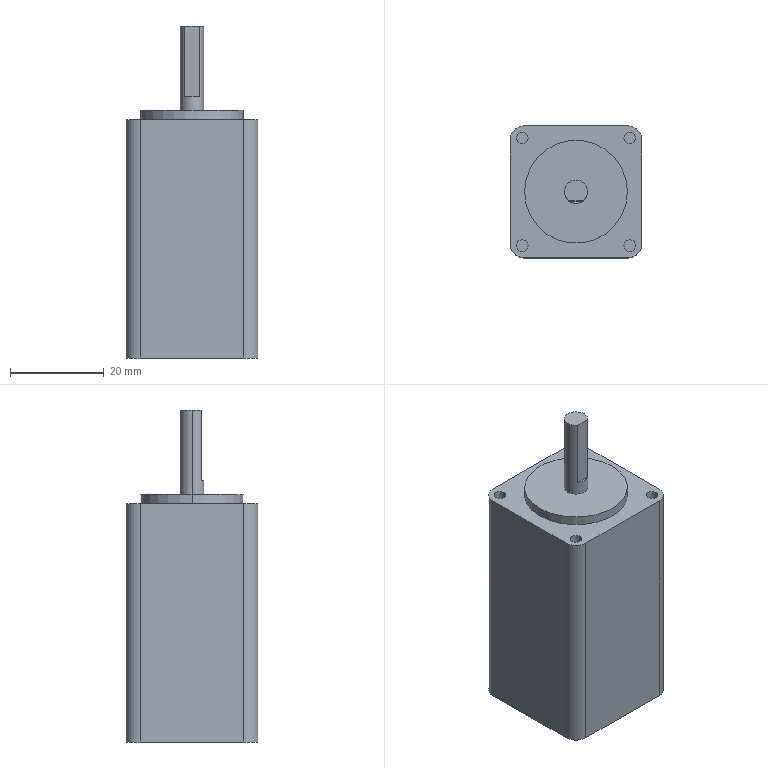Part | SolidWorks | features MBimport 1 | 1 solid | 30 faces | box 28.2 x 28.2 x 71 mm | volume 41213 mm3 | cylinder 16 | plane 14 | commonest cylinder face diameters 2.5 x8 6 x4 5 x2 22 x2
STEP:
#1=CARTESIAN_POINT('',(2.5,0.,71.));
#2=VERTEX_POINT('',#1);
#3=CARTESIAN_POINT('',(-2.5,0.,71.));
#4=VERTEX_POINT('',#3);
#5=CARTESIAN_POINT('',(0.,0.,71.));
#6=DIRECTION('',(0.,0.,1.));
#7=DIRECTION('',(1.,0.,0.));
#8=AXIS2_PLACEMENT_3D('',#5,#6,#7);
#9=CIRCLE('',#8,2.5);
#10=EDGE_CURVE('',#2,#4,#9,.T.);
#11=ORIENTED_EDGE('',*,*,#10,.F.);
#12=CARTESIAN_POINT('',(2.5,0.,53.));
#13=VERTEX_POINT('',#12);
#14=CARTESIAN_POINT('',(2.5,0.,71.));
#15=DIRECTION('',(0.,0.,-1.));
#16=VECTOR('',#15,1000.);
#17=LINE('',#14,#16);
#18=EDGE_CURVE('',#2,#13,#17,.T.);
#19=ORIENTED_EDGE('',*,*,#18,.T.);
#20=CARTESIAN_POINT('',(-2.5,0.,53.));
#21=VERTEX_POINT('',#20);
#22=CARTESIAN_POINT('',(0.,0.,53.));
#23=DIRECTION('',(0.,0.,1.));
#24=DIRECTION('',(1.,0.,0.));
#25=AXIS2_PLACEMENT_3D('',#22,#23,#24);
#26=CIRCLE('',#25,2.5);
#27=EDGE_CURVE('',#13,#21,#26,.T.);
#28=ORIENTED_EDGE('',*,*,#27,.T.);
#29=CARTESIAN_POINT('',(-2.5,0.,71.));
#30=DIRECTION('',(0.,0.,-1.));
#31=VECTOR('',#30,1000.);
#32=LINE('',#29,#31);
#33=EDGE_CURVE('',#4,#21,#32,.T.);
#34=ORIENTED_EDGE('',*,*,#33,.F.);
#35=EDGE_LOOP('',(#11,#19,#28,#34));
#36=FACE_OUTER_BOUND('',#35,.T.);
#37=CARTESIAN_POINT('',(0.,0.,71.));
#38=DIRECTION('',(0.,0.,-1.));
#39=DIRECTION('',(-1.,0.,0.));
#40=AXIS2_PLACEMENT_3D('',#37,#38,#39);
#41=CYLINDRICAL_SURFACE('',#40,2.5);
#42=ADVANCED_FACE('',(#36),#41,.T.);
#43=CARTESIAN_POINT('',(11.,0.,53.));
#44=VERTEX_POINT('',#43);
#45=CARTESIAN_POINT('',(-11.,0.,53.));
#46=VERTEX_POINT('',#45);
#47=CARTESIAN_POINT('',(0.,0.,53.));
#48=DIRECTION('',(0.,0.,1.));
#49=DIRECTION('',(1.,0.,0.));
#50=AXIS2_PLACEMENT_3D('',#47,#48,#49);
#51=CIRCLE('',#50,11.);
#52=EDGE_CURVE('',#44,#46,#51,.T.);
#53=ORIENTED_EDGE('',*,*,#52,.F.);
#54=CARTESIAN_POINT('',(11.,0.,51.));
#55=VERTEX_POINT('',#54);
#56=CARTESIAN_POINT('',(11.,0.,53.));
#57=DIRECTION('',(0.,0.,-1.));
#58=VECTOR('',#57,1000.);
#59=LINE('',#56,#58);
#60=EDGE_CURVE('',#44,#55,#59,.T.);
#61=ORIENTED_EDGE('',*,*,#60,.T.);
#62=CARTESIAN_POINT('',(-11.,0.,51.));
#63=VERTEX_POINT('',#62);
#64=CARTESIAN_POINT('',(0.,0.,51.));
#65=DIRECTION('',(0.,0.,1.));
#66=DIRECTION('',(-1.,0.,0.));
#67=AXIS2_PLACEMENT_3D('',#64,#65,#66);
#68=CIRCLE('',#67,11.);
#69=EDGE_CURVE('',#55,#63,#68,.T.);
#70=ORIENTED_EDGE('',*,*,#69,.T.);
#71=CARTESIAN_POINT('',(-11.,0.,53.));
#72=DIRECTION('',(0.,0.,-1.));
#73=VECTOR('',#72,1000.);
#74=LINE('',#71,#73);
#75=EDGE_CURVE('',#46,#63,#74,.T.);
#76=ORIENTED_EDGE('',*,*,#75,.F.);
#77=EDGE_LOOP('',(#53,#61,#70,#76));
#78=FACE_OUTER_BOUND('',#77,.T.);
#79=CARTESIAN_POINT('',(0.,0.,53.));
#80=DIRECTION('',(0.,0.,-1.));
#81=DIRECTION('',(-1.,0.,0.));
#82=AXIS2_PLACEMENT_3D('',#79,#80,#81);
#83=CYLINDRICAL_SURFACE('',#82,11.);
#84=ADVANCED_FACE('',(#78),#83,.T.);
#85=CARTESIAN_POINT('',(10.25,-11.5,48.5));
#86=VERTEX_POINT('',#85);
#87=CARTESIAN_POINT('',(12.75,-11.5,48.5));
#88=VERTEX_POINT('',#87);
#89=CARTESIAN_POINT('',(11.5,-11.5,48.5));
#90=DIRECTION('',(0.,0.,1.));
#91=DIRECTION('',(1.,0.,0.));
#92=AXIS2_PLACEMENT_3D('',#89,#90,#91);
#93=CIRCLE('',#92,1.25);
#94=EDGE_CURVE('',#86,#88,#93,.T.);
#95=ORIENTED_EDGE('',*,*,#94,.F.);
#96=CARTESIAN_POINT('',(10.25,-11.5,51.));
#97=VERTEX_POINT('',#96);
#98=CARTESIAN_POINT('',(10.25,-11.5,48.5));
#99=DIRECTION('',(0.,0.,1.));
#100=VECTOR('',#99,1000.);
#101=LINE('',#98,#100);
#102=EDGE_CURVE('',#86,#97,#101,.T.);
#103=ORIENTED_EDGE('',*,*,#102,.T.);
#104=CARTESIAN_POINT('',(12.75,-11.5,51.));
#105=VERTEX_POINT('',#104);
#106=CARTESIAN_POINT('',(11.5,-11.5,51.));
#107=DIRECTION('',(0.,0.,1.));
#108=DIRECTION('',(1.,0.,0.));
#109=AXIS2_PLACEMENT_3D('',#106,#107,#108);
#110=CIRCLE('',#109,1.25);
#111=EDGE_CURVE('',#97,#105,#110,.T.);
#112=ORIENTED_EDGE('',*,*,#111,.T.);
#113=CARTESIAN_POINT('',(12.75,-11.5,48.5));
#114=DIRECTION('',(0.,0.,1.));
#115=VECTOR('',#114,1000.);
#116=LINE('',#113,#115);
#117=EDGE_CURVE('',#88,#105,#116,.T.);
#118=ORIENTED_EDGE('',*,*,#117,.F.);
#119=EDGE_LOOP('',(#95,#103,#112,#118));
#120=FACE_OUTER_BOUND('',#119,.T.);
#121=CARTESIAN_POINT('',(11.5,-11.5,48.5));
#122=DIRECTION('',(0.,0.,1.));
#123=DIRECTION('',(1.,0.,0.));
#124=AXIS2_PLACEMENT_3D('',#121,#122,#123);
#125=CYLINDRICAL_SURFACE('',#124,1.25);
#126=ADVANCED_FACE('',(#120),#125,.F.);
#127=CARTESIAN_POINT('',(-12.75,-11.5,48.5));
#128=VERTEX_POINT('',#127);
#129=CARTESIAN_POINT('',(-10.25,-11.5,48.5));
#130=VERTEX_POINT('',#129);
#131=CARTESIAN_POINT('',(-11.5,-11.5,48.5));
#132=DIRECTION('',(0.,0.,1.));
#133=DIRECTION('',(1.,0.,0.));
#134=AXIS2_PLACEMENT_3D('',#131,#132,#133);
#135=CIRCLE('',#134,1.25);
#136=EDGE_CURVE('',#128,#130,#135,.T.);
#137=ORIENTED_EDGE('',*,*,#136,.F.);
#138=CARTESIAN_POINT('',(-12.75,-11.5,51.));
#139=VERTEX_POINT('',#138);
#140=CARTESIAN_POINT('',(-12.75,-11.5,48.5));
#141=DIRECTION('',(0.,0.,1.));
#142=VECTOR('',#141,1000.);
#143=LINE('',#140,#142);
#144=EDGE_CURVE('',#128,#139,#143,.T.);
#145=ORIENTED_EDGE('',*,*,#144,.T.);
#146=CARTESIAN_POINT('',(-10.25,-11.5,51.));
#147=VERTEX_POINT('',#146);
#148=CARTESIAN_POINT('',(-11.5,-11.5,51.));
#149=DIRECTION('',(0.,0.,1.));
#150=DIRECTION('',(1.,0.,0.));
#151=AXIS2_PLACEMENT_3D('',#148,#149,#150);
#152=CIRCLE('',#151,1.25);
#153=EDGE_CURVE('',#139,#147,#152,.T.);
#154=ORIENTED_EDGE('',*,*,#153,.T.);
#155=CARTESIAN_POINT('',(-10.25,-11.5,48.5));
#156=DIRECTION('',(0.,0.,1.));
#157=VECTOR('',#156,1000.);
#158=LINE('',#155,#157);
#159=EDGE_CURVE('',#130,#147,#158,.T.);
#160=ORIENTED_EDGE('',*,*,#159,.F.);
#161=EDGE_LOOP('',(#137,#145,#154,#160));
#162=FACE_OUTER_BOUND('',#161,.T.);
#163=CARTESIAN_POINT('',(-11.5,-11.5,48.5));
#164=DIRECTION('',(0.,0.,1.));
#165=DIRECTION('',(1.,0.,0.));
#166=AXIS2_PLACEMENT_3D('',#163,#164,#165);
#167=CYLINDRICAL_SURFACE('',#166,1.25);
#168=ADVANCED_FACE('',(#162),#167,.F.);
#169=CARTESIAN_POINT('',(10.25,11.5,48.5));
#170=VERTEX_POINT('',#169);
#171=CARTESIAN_POINT('',(12.75,11.5,48.5));
#172=VERTEX_POINT('',#171);
#173=CARTESIAN_POINT('',(11.5,11.5,48.5));
#174=DIRECTION('',(0.,0.,1.));
#175=DIRECTION('',(1.,0.,0.));
#176=AXIS2_PLACEMENT_3D('',#173,#174,#175);
#177=CIRCLE('',#176,1.25);
#178=EDGE_CURVE('',#170,#172,#177,.T.);
#179=ORIENTED_EDGE('',*,*,#178,.F.);
#180=CARTESIAN_POINT('',(10.25,11.5,51.));
#181=VERTEX_POINT('',#180);
#182=CARTESIAN_POINT('',(10.25,11.5,48.5));
#183=DIRECTION('',(0.,0.,1.));
#184=VECTOR('',#183,1000.);
#185=LINE('',#182,#184);
#186=EDGE_CURVE('',#170,#181,#185,.T.);
#187=ORIENTED_EDGE('',*,*,#186,.T.);
#188=CARTESIAN_POINT('',(12.75,11.5,51.));
#189=VERTEX_POINT('',#188);
#190=CARTESIAN_POINT('',(11.5,11.5,51.));
#191=DIRECTION('',(0.,0.,1.));
#192=DIRECTION('',(1.,0.,0.));
#193=AXIS2_PLACEMENT_3D('',#190,#191,#192);
#194=CIRCLE('',#193,1.25);
#195=EDGE_CURVE('',#181,#189,#194,.T.);
#196=ORIENTED_EDGE('',*,*,#195,.T.);
#197=CARTESIAN_POINT('',(12.75,11.5,48.5));
#198=DIRECTION('',(0.,0.,1.));
#199=VECTOR('',#198,1000.);
#200=LINE('',#197,#199);
#201=EDGE_CURVE('',#172,#189,#200,.T.);
#202=ORIENTED_EDGE('',*,*,#201,.F.);
#203=EDGE_LOOP('',(#179,#187,#196,#202));
#204=FACE_OUTER_BOUND('',#203,.T.);
#205=CARTESIAN_POINT('',(11.5,11.5,48.5));
#206=DIRECTION('',(0.,0.,1.));
#207=DIRECTION('',(1.,0.,0.));
#208=AXIS2_PLACEMENT_3D('',#205,#206,#207);
#209=CYLINDRICAL_SURFACE('',#208,1.25);
#210=ADVANCED_FACE('',(#204),#209,.F.);
#211=CARTESIAN_POINT('',(-12.75,11.5,48.5));
#212=VERTEX_POINT('',#211);
#213=CARTESIAN_POINT('',(-10.25,11.5,48.5));
#214=VERTEX_POINT('',#213);
#215=CARTESIAN_POINT('',(-11.5,11.5,48.5));
#216=DIRECTION('',(0.,0.,1.));
#217=DIRECTION('',(1.,0.,0.));
#218=AXIS2_PLACEMENT_3D('',#215,#216,#217);
#219=CIRCLE('',#218,1.25);
#220=EDGE_CURVE('',#212,#214,#219,.T.);
#221=ORIENTED_EDGE('',*,*,#220,.F.);
#222=CARTESIAN_POINT('',(-12.75,11.5,51.));
#223=VERTEX_POINT('',#222);
#224=CARTESIAN_POINT('',(-12.75,11.5,48.5));
#225=DIRECTION('',(0.,0.,1.));
#226=VECTOR('',#225,1000.);
#227=LINE('',#224,#226);
#228=EDGE_CURVE('',#212,#223,#227,.T.);
#229=ORIENTED_EDGE('',*,*,#228,.T.);
#230=CARTESIAN_POINT('',(-10.25,11.5,51.));
#231=VERTEX_POINT('',#230);
#232=CARTESIAN_POINT('',(-11.5,11.5,51.));
#233=DIRECTION('',(0.,0.,1.));
#234=DIRECTION('',(1.,0.,0.));
#235=AXIS2_PLACEMENT_3D('',#232,#233,#234);
#236=CIRCLE('',#235,1.25);
#237=EDGE_CURVE('',#223,#231,#236,.T.);
#238=ORIENTED_EDGE('',*,*,#237,.T.);
#239=CARTESIAN_POINT('',(-10.25,11.5,48.5));
#240=DIRECTION('',(0.,0.,1.));
#241=VECTOR('',#240,1000.);
#242=LINE('',#239,#241);
#243=EDGE_CURVE('',#214,#231,#242,.T.);
#244=ORIENTED_EDGE('',*,*,#243,.F.);
#245=EDGE_LOOP('',(#221,#229,#238,#244));
#246=FACE_OUTER_BOUND('',#245,.T.);
#247=CARTESIAN_POINT('',(-11.5,11.5,48.5));
#248=DIRECTION('',(0.,0.,1.));
#249=DIRECTION('',(1.,0.,0.));
#250=AXIS2_PLACEMENT_3D('',#247,#248,#249);
#251=CYLINDRICAL_SURFACE('',#250,1.25);
#252=ADVANCED_FACE('',(#246),#251,.F.);
#253=CARTESIAN_POINT('',(0.,0.,53.));
#254=DIRECTION('',(0.,0.,1.));
#255=DIRECTION('',(1.,0.,0.));
#256=AXIS2_PLACEMENT_3D('',#253,#254,#255);
#257=CIRCLE('',#256,11.);
#258=EDGE_CURVE('',#46,#44,#257,.T.);
#259=ORIENTED_EDGE('',*,*,#258,.T.);
#260=ORIENTED_EDGE('',*,*,#52,.T.);
#261=EDGE_LOOP('',(#259,#260));
#262=FACE_OUTER_BOUND('',#261,.T.);
#263=CARTESIAN_POINT('',(0.,0.,53.));
#264=DIRECTION('',(0.,0.,1.));
#265=DIRECTION('',(1.,0.,0.));
#266=AXIS2_PLACEMENT_3D('',#263,#264,#265);
#267=CIRCLE('',#266,2.5);
#268=EDGE_CURVE('',#21,#13,#267,.T.);
#269=ORIENTED_EDGE('',*,*,#268,.F.);
#270=ORIENTED_EDGE('',*,*,#27,.F.);
#271=EDGE_LOOP('',(#269,#270));
#272=FACE_BOUND('',#271,.T.);
#273=CARTESIAN_POINT('',(0.,0.,53.));
#274=DIRECTION('',(0.,0.,1.));
#275=DIRECTION('',(1.,0.,0.));
#276=AXIS2_PLACEMENT_3D('',#273,#274,#275);
#277=PLANE('',#276);
#278=ADVANCED_FACE('',(#262,#272),#277,.T.);
#279=CARTESIAN_POINT('',(-14.1,11.1,51.));
#280=VERTEX_POINT('',#279);
#281=CARTESIAN_POINT('',(-14.1,-11.1,51.));
#282=VERTEX_POINT('',#281);
#283=CARTESIAN_POINT('',(-14.1,-14.1,51.));
#284=DIRECTION('',(0.,-1.,0.));
#285=VECTOR('',#284,1000.);
#286=LINE('',#283,#285);
#287=EDGE_CURVE('',#280,#282,#286,.T.);
#288=ORIENTED_EDGE('',*,*,#287,.T.);
#289=CARTESIAN_POINT('',(-11.1,-14.1,51.));
#290=VERTEX_POINT('',#289);
#291=CARTESIAN_POINT('',(-11.1,-11.1,51.));
#292=DIRECTION('',(0.,0.,1.));
#293=DIRECTION('',(-1.,0.,0.));
#294=AXIS2_PLACEMENT_3D('',#291,#292,#293);
#295=CIRCLE('',#294,3.);
#296=EDGE_CURVE('',#282,#290,#295,.T.);
#297=ORIENTED_EDGE('',*,*,#296,.T.);
#298=CARTESIAN_POINT('',(11.1,-14.1,51.));
#299=VERTEX_POINT('',#298);
#300=CARTESIAN_POINT('',(-14.1,-14.1,51.));
#301=DIRECTION('',(1.,0.,0.));
#302=VECTOR('',#301,1000.);
#303=LINE('',#300,#302);
#304=EDGE_CURVE('',#290,#299,#303,.T.);
#305=ORIENTED_EDGE('',*,*,#304,.T.);
#306=CARTESIAN_POINT('',(14.1,-11.1,51.));
#307=VERTEX_POINT('',#306);
#308=CARTESIAN_POINT('',(11.1,-11.1,51.));
#309=DIRECTION('',(0.,0.,1.));
#310=DIRECTION('',(-1.,0.,0.));
#311=AXIS2_PLACEMENT_3D('',#308,#309,#310);
#312=CIRCLE('',#311,3.);
#313=EDGE_CURVE('',#299,#307,#312,.T.);
#314=ORIENTED_EDGE('',*,*,#313,.T.);
#315=CARTESIAN_POINT('',(14.1,11.1,51.));
#316=VERTEX_POINT('',#315);
#317=CARTESIAN_POINT('',(14.1,-14.1,51.));
#318=DIRECTION('',(0.,1.,0.));
#319=VECTOR('',#318,1000.);
#320=LINE('',#317,#319);
#321=EDGE_CURVE('',#307,#316,#320,.T.);
#322=ORIENTED_EDGE('',*,*,#321,.T.);
#323=CARTESIAN_POINT('',(11.1,14.1,51.));
#324=VERTEX_POINT('',#323);
#325=CARTESIAN_POINT('',(11.1,11.1,51.));
#326=DIRECTION('',(0.,0.,1.));
#327=DIRECTION('',(-1.,0.,0.));
#328=AXIS2_PLACEMENT_3D('',#325,#326,#327);
#329=CIRCLE('',#328,3.);
#330=EDGE_CURVE('',#316,#324,#329,.T.);
#331=ORIENTED_EDGE('',*,*,#330,.T.);
#332=CARTESIAN_POINT('',(-11.1,14.1,51.));
#333=VERTEX_POINT('',#332);
#334=CARTESIAN_POINT('',(-14.1,14.1,51.));
#335=DIRECTION('',(-1.,0.,0.));
#336=VECTOR('',#335,1000.);
#337=LINE('',#334,#336);
#338=EDGE_CURVE('',#324,#333,#337,.T.);
#339=ORIENTED_EDGE('',*,*,#338,.T.);
#340=CARTESIAN_POINT('',(-11.1,11.1,51.));
#341=DIRECTION('',(0.,0.,1.));
#342=DIRECTION('',(-1.,0.,0.));
#343=AXIS2_PLACEMENT_3D('',#340,#341,#342);
#344=CIRCLE('',#343,3.);
#345=EDGE_CURVE('',#333,#280,#344,.T.);
#346=ORIENTED_EDGE('',*,*,#345,.T.);
#347=EDGE_LOOP('',(#288,#297,#305,#314,#322,#331,#339,#346));
#348=FACE_OUTER_BOUND('',#347,.T.);
#349=CARTESIAN_POINT('',(-11.5,11.5,51.));
#350=DIRECTION('',(0.,0.,1.));
#351=DIRECTION('',(1.,0.,0.));
#352=AXIS2_PLACEMENT_3D('',#349,#350,#351);
#353=CIRCLE('',#352,1.25);
#354=EDGE_CURVE('',#231,#223,#353,.T.);
#355=ORIENTED_EDGE('',*,*,#354,.F.);
#356=ORIENTED_EDGE('',*,*,#237,.F.);
#357=EDGE_LOOP('',(#355,#356));
#358=FACE_BOUND('',#357,.T.);
#359=CARTESIAN_POINT('',(11.5,11.5,51.));
#360=DIRECTION('',(0.,0.,1.));
#361=DIRECTION('',(1.,0.,0.));
#362=AXIS2_PLACEMENT_3D('',#359,#360,#361);
#363=CIRCLE('',#362,1.25);
#364=EDGE_CURVE('',#189,#181,#363,.T.);
#365=ORIENTED_EDGE('',*,*,#364,.F.);
#366=ORIENTED_EDGE('',*,*,#195,.F.);
#367=EDGE_LOOP('',(#365,#366));
#368=FACE_BOUND('',#367,.T.);
#369=CARTESIAN_POINT('',(-11.5,-11.5,51.));
#370=DIRECTION('',(0.,0.,1.));
#371=DIRECTION('',(1.,0.,0.));
#372=AXIS2_PLACEMENT_3D('',#369,#370,#371);
#373=CIRCLE('',#372,1.25);
#374=EDGE_CURVE('',#147,#139,#373,.T.);
#375=ORIENTED_EDGE('',*,*,#374,.F.);
#376=ORIENTED_EDGE('',*,*,#153,.F.);
#377=EDGE_LOOP('',(#375,#376));
#378=FACE_BOUND('',#377,.T.);
#379=CARTESIAN_POINT('',(11.5,-11.5,51.));
#380=DIRECTION('',(0.,0.,1.));
#381=DIRECTION('',(1.,0.,0.));
#382=AXIS2_PLACEMENT_3D('',#379,#380,#381);
#383=CIRCLE('',#382,1.25);
#384=EDGE_CURVE('',#105,#97,#383,.T.);
#385=ORIENTED_EDGE('',*,*,#384,.F.);
#386=ORIENTED_EDGE('',*,*,#111,.F.);
#387=EDGE_LOOP('',(#385,#386));
#388=FACE_BOUND('',#387,.T.);
#389=CARTESIAN_POINT('',(0.,0.,51.));
#390=DIRECTION('',(0.,0.,1.));
#391=DIRECTION('',(-1.,0.,0.));
#392=AXIS2_PLACEMENT_3D('',#389,#390,#391);
#393=CIRCLE('',#392,11.);
#394=EDGE_CURVE('',#63,#55,#393,.T.);
#395=ORIENTED_EDGE('',*,*,#394,.F.);
#396=ORIENTED_EDGE('',*,*,#69,.F.);
#397=EDGE_LOOP('',(#395,#396));
#398=FACE_BOUND('',#397,.T.);
#399=CARTESIAN_POINT('',(14.1,14.1,51.));
#400=DIRECTION('',(0.,0.,-1.));
#401=DIRECTION('',(0.,-1.,0.));
#402=AXIS2_PLACEMENT_3D('',#399,#400,#401);
#403=PLANE('',#402);
#404=ADVANCED_FACE('',(#348,#358,#368,#378,#388,#398),#403,.F.);
#405=CARTESIAN_POINT('',(14.1,-11.1,0.));
#406=VERTEX_POINT('',#405);
#407=CARTESIAN_POINT('',(14.1,11.1,0.));
#408=VERTEX_POINT('',#407);
#409=CARTESIAN_POINT('',(14.1,-14.1,0.));
#410=DIRECTION('',(0.,1.,0.));
#411=VECTOR('',#410,1000.);
#412=LINE('',#409,#411);
#413=EDGE_CURVE('',#406,#408,#412,.T.);
#414=ORIENTED_EDGE('',*,*,#413,.T.);
#415=CARTESIAN_POINT('',(14.1,11.1,51.));
#416=DIRECTION('',(0.,0.,1.));
#417=VECTOR('',#416,1000.);
#418=LINE('',#415,#417);
#419=EDGE_CURVE('',#408,#316,#418,.T.);
#420=ORIENTED_EDGE('',*,*,#419,.T.);
#421=ORIENTED_EDGE('',*,*,#321,.F.);
#422=CARTESIAN_POINT('',(14.1,-11.1,51.));
#423=DIRECTION('',(0.,0.,-1.));
#424=VECTOR('',#423,1000.);
#425=LINE('',#422,#424);
#426=EDGE_CURVE('',#307,#406,#425,.T.);
#427=ORIENTED_EDGE('',*,*,#426,.T.);
#428=EDGE_LOOP('',(#414,#420,#421,#427));
#429=FACE_OUTER_BOUND('',#428,.T.);
#430=CARTESIAN_POINT('',(14.1,-14.1,51.));
#431=DIRECTION('',(-1.,0.,0.));
#432=DIRECTION('',(0.,0.,1.));
#433=AXIS2_PLACEMENT_3D('',#430,#431,#432);
#434=PLANE('',#433);
#435=ADVANCED_FACE('',(#429),#434,.F.);
#436=CARTESIAN_POINT('',(11.1,14.1,0.));
#437=VERTEX_POINT('',#436);
#438=CARTESIAN_POINT('',(-11.1,14.1,0.));
#439=VERTEX_POINT('',#438);
#440=CARTESIAN_POINT('',(-14.1,14.1,0.));
#441=DIRECTION('',(-1.,0.,0.));
#442=VECTOR('',#441,1000.);
#443=LINE('',#440,#442);
#444=EDGE_CURVE('',#437,#439,#443,.T.);
#445=ORIENTED_EDGE('',*,*,#444,.T.);
#446=CARTESIAN_POINT('',(-11.1,14.1,51.));
#447=DIRECTION('',(0.,0.,1.));
#448=VECTOR('',#447,1000.);
#449=LINE('',#446,#448);
#450=EDGE_CURVE('',#439,#333,#449,.T.);
#451=ORIENTED_EDGE('',*,*,#450,.T.);
#452=ORIENTED_EDGE('',*,*,#338,.F.);
#453=CARTESIAN_POINT('',(11.1,14.1,51.));
#454=DIRECTION('',(0.,0.,-1.));
#455=VECTOR('',#454,1000.);
#456=LINE('',#453,#455);
#457=EDGE_CURVE('',#324,#437,#456,.T.);
#458=ORIENTED_EDGE('',*,*,#457,.T.);
#459=EDGE_LOOP('',(#445,#451,#452,#458));
#460=FACE_OUTER_BOUND('',#459,.T.);
#461=CARTESIAN_POINT('',(-14.1,14.1,51.));
#462=DIRECTION('',(0.,-1.,0.));
#463=DIRECTION('',(0.,0.,-1.));
#464=AXIS2_PLACEMENT_3D('',#461,#462,#463);
#465=PLANE('',#464);
#466=ADVANCED_FACE('',(#460),#465,.F.);
#467=CARTESIAN_POINT('',(-14.1,11.1,0.));
#468=VERTEX_POINT('',#467);
#469=CARTESIAN_POINT('',(-14.1,-11.1,0.));
#470=VERTEX_POINT('',#469);
#471=CARTESIAN_POINT('',(-14.1,-14.1,0.));
#472=DIRECTION('',(0.,-1.,0.));
#473=VECTOR('',#472,1000.);
#474=LINE('',#471,#473);
#475=EDGE_CURVE('',#468,#470,#474,.T.);
#476=ORIENTED_EDGE('',*,*,#475,.T.);
#477=CARTESIAN_POINT('',(-14.1,-11.1,51.));
#478=DIRECTION('',(0.,0.,1.));
#479=VECTOR('',#478,1000.);
#480=LINE('',#477,#479);
#481=EDGE_CURVE('',#470,#282,#480,.T.);
#482=ORIENTED_EDGE('',*,*,#481,.T.);
#483=ORIENTED_EDGE('',*,*,#287,.F.);
#484=CARTESIAN_POINT('',(-14.1,11.1,51.));
#485=DIRECTION('',(0.,0.,-1.));
#486=VECTOR('',#485,1000.);
#487=LINE('',#484,#486);
#488=EDGE_CURVE('',#280,#468,#487,.T.);
#489=ORIENTED_EDGE('',*,*,#488,.T.);
#490=EDGE_LOOP('',(#476,#482,#483,#489));
#491=FACE_OUTER_BOUND('',#490,.T.);
#492=CARTESIAN_POINT('',(-14.1,-14.1,51.));
#493=DIRECTION('',(1.,0.,0.));
#494=DIRECTION('',(0.,1.,0.));
#495=AXIS2_PLACEMENT_3D('',#492,#493,#494);
#496=PLANE('',#495);
#497=ADVANCED_FACE('',(#491),#496,.F.);
#498=ORIENTED_EDGE('',*,*,#304,.F.);
#499=CARTESIAN_POINT('',(-11.1,-14.1,0.));
#500=VERTEX_POINT('',#499);
#501=CARTESIAN_POINT('',(-11.1,-14.1,51.));
#502=DIRECTION('',(0.,0.,-1.));
#503=VECTOR('',#502,1000.);
#504=LINE('',#501,#503);
#505=EDGE_CURVE('',#290,#500,#504,.T.);
#506=ORIENTED_EDGE('',*,*,#505,.T.);
#507=CARTESIAN_POINT('',(11.1,-14.1,0.));
#508=VERTEX_POINT('',#507);
#509=CARTESIAN_POINT('',(-14.1,-14.1,0.));
#510=DIRECTION('',(1.,0.,0.));
#511=VECTOR('',#510,1000.);
#512=LINE('',#509,#511);
#513=EDGE_CURVE('',#500,#508,#512,.T.);
#514=ORIENTED_EDGE('',*,*,#513,.T.);
#515=CARTESIAN_POINT('',(11.1,-14.1,51.));
#516=DIRECTION('',(0.,0.,1.));
#517=VECTOR('',#516,1000.);
#518=LINE('',#515,#517);
#519=EDGE_CURVE('',#508,#299,#518,.T.);
#520=ORIENTED_EDGE('',*,*,#519,.T.);
#521=EDGE_LOOP('',(#498,#506,#514,#520));
#522=FACE_OUTER_BOUND('',#521,.T.);
#523=CARTESIAN_POINT('',(-14.1,-14.1,51.));
#524=DIRECTION('',(0.,1.,0.));
#525=DIRECTION('',(1.,0.,0.));
#526=AXIS2_PLACEMENT_3D('',#523,#524,#525);
#527=PLANE('',#526);
#528=ADVANCED_FACE('',(#522),#527,.F.);
#529=ORIENTED_EDGE('',*,*,#513,.F.);
#530=CARTESIAN_POINT('',(-11.1,-11.1,0.));
#531=DIRECTION('',(0.,0.,-1.));
#532=DIRECTION('',(-1.,0.,0.));
#533=AXIS2_PLACEMENT_3D('',#530,#531,#532);
#534=CIRCLE('',#533,3.);
#535=EDGE_CURVE('',#500,#470,#534,.T.);
#536=ORIENTED_EDGE('',*,*,#535,.T.);
#537=ORIENTED_EDGE('',*,*,#475,.F.);
#538=CARTESIAN_POINT('',(-11.1,11.1,0.));
#539=DIRECTION('',(0.,0.,-1.));
#540=DIRECTION('',(-1.,0.,0.));
#541=AXIS2_PLACEMENT_3D('',#538,#539,#540);
#542=CIRCLE('',#541,3.);
#543=EDGE_CURVE('',#468,#439,#542,.T.);
#544=ORIENTED_EDGE('',*,*,#543,.T.);
#545=ORIENTED_EDGE('',*,*,#444,.F.);
#546=CARTESIAN_POINT('',(11.1,11.1,0.));
#547=DIRECTION('',(0.,0.,-1.));
#548=DIRECTION('',(-1.,0.,0.));
#549=AXIS2_PLACEMENT_3D('',#546,#547,#548);
#550=CIRCLE('',#549,3.);
#551=EDGE_CURVE('',#437,#408,#550,.T.);
#552=ORIENTED_EDGE('',*,*,#551,.T.);
#553=ORIENTED_EDGE('',*,*,#413,.F.);
#554=CARTESIAN_POINT('',(11.1,-11.1,0.));
#555=DIRECTION('',(0.,0.,-1.));
#556=DIRECTION('',(-1.,0.,0.));
#557=AXIS2_PLACEMENT_3D('',#554,#555,#556);
#558=CIRCLE('',#557,3.);
#559=EDGE_CURVE('',#406,#508,#558,.T.);
#560=ORIENTED_EDGE('',*,*,#559,.T.);
#561=EDGE_LOOP('',(#529,#536,#537,#544,#545,#552,#553,#560));
#562=FACE_OUTER_BOUND('',#561,.T.);
#563=CARTESIAN_POINT('',(14.1,14.1,0.));
#564=DIRECTION('',(0.,0.,-1.));
#565=DIRECTION('',(0.,-1.,0.));
#566=AXIS2_PLACEMENT_3D('',#563,#564,#565);
#567=PLANE('',#566);
#568=ADVANCED_FACE('',(#562),#567,.T.);
#569=ORIENTED_EDGE('',*,*,#228,.F.);
#570=CARTESIAN_POINT('',(-11.5,11.5,48.5));
#571=DIRECTION('',(0.,0.,1.));
#572=DIRECTION('',(1.,0.,0.));
#573=AXIS2_PLACEMENT_3D('',#570,#571,#572);
#574=CIRCLE('',#573,1.25);
#575=EDGE_CURVE('',#214,#212,#574,.T.);
#576=ORIENTED_EDGE('',*,*,#575,.F.);
#577=ORIENTED_EDGE('',*,*,#243,.T.);
#578=ORIENTED_EDGE('',*,*,#354,.T.);
#579=EDGE_LOOP('',(#569,#576,#577,#578));
#580=FACE_OUTER_BOUND('',#579,.T.);
#581=CARTESIAN_POINT('',(-11.5,11.5,48.5));
#582=DIRECTION('',(0.,0.,1.));
#583=DIRECTION('',(1.,0.,0.));
#584=AXIS2_PLACEMENT_3D('',#581,#582,#583);
#585=CYLINDRICAL_SURFACE('',#584,1.25);
#586=ADVANCED_FACE('',(#580),#585,.F.);
#587=ORIENTED_EDGE('',*,*,#575,.T.);
#588=ORIENTED_EDGE('',*,*,#220,.T.);
#589=EDGE_LOOP('',(#587,#588));
#590=FACE_OUTER_BOUND('',#589,.T.);
#591=CARTESIAN_POINT('',(-11.5,11.5,48.5));
#592=DIRECTION('',(0.,0.,1.));
#593=DIRECTION('',(1.,0.,0.));
#594=AXIS2_PLACEMENT_3D('',#591,#592,#593);
#595=PLANE('',#594);
#596=ADVANCED_FACE('',(#590),#595,.T.);
#597=ORIENTED_EDGE('',*,*,#186,.F.);
#598=CARTESIAN_POINT('',(11.5,11.5,48.5));
#599=DIRECTION('',(0.,0.,1.));
#600=DIRECTION('',(1.,0.,0.));
#601=AXIS2_PLACEMENT_3D('',#598,#599,#600);
#602=CIRCLE('',#601,1.25);
#603=EDGE_CURVE('',#172,#170,#602,.T.);
#604=ORIENTED_EDGE('',*,*,#603,.F.);
#605=ORIENTED_EDGE('',*,*,#201,.T.);
#606=ORIENTED_EDGE('',*,*,#364,.T.);
#607=EDGE_LOOP('',(#597,#604,#605,#606));
#608=FACE_OUTER_BOUND('',#607,.T.);
#609=CARTESIAN_POINT('',(11.5,11.5,48.5));
#610=DIRECTION('',(0.,0.,1.));
#611=DIRECTION('',(1.,0.,0.));
#612=AXIS2_PLACEMENT_3D('',#609,#610,#611);
#613=CYLINDRICAL_SURFACE('',#612,1.25);
#614=ADVANCED_FACE('',(#608),#613,.F.);
#615=ORIENTED_EDGE('',*,*,#603,.T.);
#616=ORIENTED_EDGE('',*,*,#178,.T.);
#617=EDGE_LOOP('',(#615,#616));
#618=FACE_OUTER_BOUND('',#617,.T.);
#619=CARTESIAN_POINT('',(11.5,11.5,48.5));
#620=DIRECTION('',(0.,0.,1.));
#621=DIRECTION('',(1.,0.,0.));
#622=AXIS2_PLACEMENT_3D('',#619,#620,#621);
#623=PLANE('',#622);
#624=ADVANCED_FACE('',(#618),#623,.T.);
#625=ORIENTED_EDGE('',*,*,#144,.F.);
#626=CARTESIAN_POINT('',(-11.5,-11.5,48.5));
#627=DIRECTION('',(0.,0.,1.));
#628=DIRECTION('',(1.,0.,0.));
#629=AXIS2_PLACEMENT_3D('',#626,#627,#628);
#630=CIRCLE('',#629,1.25);
#631=EDGE_CURVE('',#130,#128,#630,.T.);
#632=ORIENTED_EDGE('',*,*,#631,.F.);
#633=ORIENTED_EDGE('',*,*,#159,.T.);
#634=ORIENTED_EDGE('',*,*,#374,.T.);
#635=EDGE_LOOP('',(#625,#632,#633,#634));
#636=FACE_OUTER_BOUND('',#635,.T.);
#637=CARTESIAN_POINT('',(-11.5,-11.5,48.5));
#638=DIRECTION('',(0.,0.,1.));
#639=DIRECTION('',(1.,0.,0.));
#640=AXIS2_PLACEMENT_3D('',#637,#638,#639);
#641=CYLINDRICAL_SURFACE('',#640,1.25);
#642=ADVANCED_FACE('',(#636),#641,.F.);
#643=ORIENTED_EDGE('',*,*,#631,.T.);
#644=ORIENTED_EDGE('',*,*,#136,.T.);
#645=EDGE_LOOP('',(#643,#644));
#646=FACE_OUTER_BOUND('',#645,.T.);
#647=CARTESIAN_POINT('',(-11.5,-11.5,48.5));
#648=DIRECTION('',(0.,0.,1.));
#649=DIRECTION('',(1.,0.,0.));
#650=AXIS2_PLACEMENT_3D('',#647,#648,#649);
#651=PLANE('',#650);
#652=ADVANCED_FACE('',(#646),#651,.T.);
#653=ORIENTED_EDGE('',*,*,#102,.F.);
#654=CARTESIAN_POINT('',(11.5,-11.5,48.5));
#655=DIRECTION('',(0.,0.,1.));
#656=DIRECTION('',(1.,0.,0.));
#657=AXIS2_PLACEMENT_3D('',#654,#655,#656);
#658=CIRCLE('',#657,1.25);
#659=EDGE_CURVE('',#88,#86,#658,.T.);
#660=ORIENTED_EDGE('',*,*,#659,.F.);
#661=ORIENTED_EDGE('',*,*,#117,.T.);
#662=ORIENTED_EDGE('',*,*,#384,.T.);
#663=EDGE_LOOP('',(#653,#660,#661,#662));
#664=FACE_OUTER_BOUND('',#663,.T.);
#665=CARTESIAN_POINT('',(11.5,-11.5,48.5));
#666=DIRECTION('',(0.,0.,1.));
#667=DIRECTION('',(1.,0.,0.));
#668=AXIS2_PLACEMENT_3D('',#665,#666,#667);
#669=CYLINDRICAL_SURFACE('',#668,1.25);
#670=ADVANCED_FACE('',(#664),#669,.F.);
#671=ORIENTED_EDGE('',*,*,#659,.T.);
#672=ORIENTED_EDGE('',*,*,#94,.T.);
#673=EDGE_LOOP('',(#671,#672));
#674=FACE_OUTER_BOUND('',#673,.T.);
#675=CARTESIAN_POINT('',(11.5,-11.5,48.5));
#676=DIRECTION('',(0.,0.,1.));
#677=DIRECTION('',(1.,0.,0.));
#678=AXIS2_PLACEMENT_3D('',#675,#676,#677);
#679=PLANE('',#678);
#680=ADVANCED_FACE('',(#674),#679,.T.);
#681=ORIENTED_EDGE('',*,*,#60,.F.);
#682=ORIENTED_EDGE('',*,*,#258,.F.);
#683=ORIENTED_EDGE('',*,*,#75,.T.);
#684=ORIENTED_EDGE('',*,*,#394,.T.);
#685=EDGE_LOOP('',(#681,#682,#683,#684));
#686=FACE_OUTER_BOUND('',#685,.T.);
#687=CARTESIAN_POINT('',(0.,0.,53.));
#688=DIRECTION('',(0.,0.,-1.));
#689=DIRECTION('',(-1.,0.,0.));
#690=AXIS2_PLACEMENT_3D('',#687,#688,#689);
#691=CYLINDRICAL_SURFACE('',#690,11.);
#692=ADVANCED_FACE('',(#686),#691,.T.);
#693=ORIENTED_EDGE('',*,*,#18,.F.);
#694=CARTESIAN_POINT('',(1.5,-2.,71.));
#695=VERTEX_POINT('',#694);
#696=CARTESIAN_POINT('',(0.,0.,71.));
#697=DIRECTION('',(0.,0.,1.));
#698=DIRECTION('',(1.,0.,0.));
#699=AXIS2_PLACEMENT_3D('',#696,#697,#698);
#700=CIRCLE('',#699,2.5);
#701=EDGE_CURVE('',#695,#2,#700,.T.);
#702=ORIENTED_EDGE('',*,*,#701,.F.);
#703=CARTESIAN_POINT('',(1.5,-2.,56.));
#704=VERTEX_POINT('',#703);
#705=CARTESIAN_POINT('',(1.5,-2.,71.));
#706=DIRECTION('',(0.,0.,-1.));
#707=VECTOR('',#706,1000.);
#708=LINE('',#705,#707);
#709=EDGE_CURVE('',#695,#704,#708,.T.);
#710=ORIENTED_EDGE('',*,*,#709,.T.);
#711=CARTESIAN_POINT('',(-1.5,-2.,56.));
#712=VERTEX_POINT('',#711);
#713=CARTESIAN_POINT('',(0.,0.,56.));
#714=DIRECTION('',(0.,0.,1.));
#715=DIRECTION('',(1.,0.,0.));
#716=AXIS2_PLACEMENT_3D('',#713,#714,#715);
#717=CIRCLE('',#716,2.5);
#718=EDGE_CURVE('',#712,#704,#717,.T.);
#719=ORIENTED_EDGE('',*,*,#718,.F.);
#720=CARTESIAN_POINT('',(-1.5,-2.,71.));
#721=VERTEX_POINT('',#720);
#722=CARTESIAN_POINT('',(-1.5,-2.,71.));
#723=DIRECTION('',(0.,0.,1.));
#724=VECTOR('',#723,1000.);
#725=LINE('',#722,#724);
#726=EDGE_CURVE('',#712,#721,#725,.T.);
#727=ORIENTED_EDGE('',*,*,#726,.T.);
#728=CARTESIAN_POINT('',(0.,0.,71.));
#729=DIRECTION('',(0.,0.,1.));
#730=DIRECTION('',(1.,0.,0.));
#731=AXIS2_PLACEMENT_3D('',#728,#729,#730);
#732=CIRCLE('',#731,2.5);
#733=EDGE_CURVE('',#4,#721,#732,.T.);
#734=ORIENTED_EDGE('',*,*,#733,.F.);
#735=ORIENTED_EDGE('',*,*,#33,.T.);
#736=ORIENTED_EDGE('',*,*,#268,.T.);
#737=EDGE_LOOP('',(#693,#702,#710,#719,#727,#734,#735,#736));
#738=FACE_OUTER_BOUND('',#737,.T.);
#739=CARTESIAN_POINT('',(0.,0.,71.));
#740=DIRECTION('',(0.,0.,-1.));
#741=DIRECTION('',(-1.,0.,0.));
#742=AXIS2_PLACEMENT_3D('',#739,#740,#741);
#743=CYLINDRICAL_SURFACE('',#742,2.5);
#744=ADVANCED_FACE('',(#738),#743,.T.);
#745=CARTESIAN_POINT('',(0.,-2.,71.));
#746=DIRECTION('',(-1.,0.,0.));
#747=VECTOR('',#746,1000.);
#748=LINE('',#745,#747);
#749=EDGE_CURVE('',#695,#721,#748,.T.);
#750=ORIENTED_EDGE('',*,*,#749,.F.);
#751=ORIENTED_EDGE('',*,*,#701,.T.);
#752=ORIENTED_EDGE('',*,*,#10,.T.);
#753=ORIENTED_EDGE('',*,*,#733,.T.);
#754=EDGE_LOOP('',(#750,#751,#752,#753));
#755=FACE_OUTER_BOUND('',#754,.T.);
#756=CARTESIAN_POINT('',(0.,0.,71.));
#757=DIRECTION('',(0.,0.,1.));
#758=DIRECTION('',(1.,0.,0.));
#759=AXIS2_PLACEMENT_3D('',#756,#757,#758);
#760=PLANE('',#759);
#761=ADVANCED_FACE('',(#755),#760,.T.);
#762=ORIENTED_EDGE('',*,*,#718,.T.);
#763=CARTESIAN_POINT('',(0.,-2.,56.));
#764=DIRECTION('',(-1.,0.,0.));
#765=VECTOR('',#764,1000.);
#766=LINE('',#763,#765);
#767=EDGE_CURVE('',#704,#712,#766,.T.);
#768=ORIENTED_EDGE('',*,*,#767,.T.);
#769=EDGE_LOOP('',(#762,#768));
#770=FACE_OUTER_BOUND('',#769,.T.);
#771=CARTESIAN_POINT('',(7.156,-2.,56.));
#772=DIRECTION('',(0.,0.,1.));
#773=DIRECTION('',(1.,0.,0.));
#774=AXIS2_PLACEMENT_3D('',#771,#772,#773);
#775=PLANE('',#774);
#776=ADVANCED_FACE('',(#770),#775,.T.);
#777=ORIENTED_EDGE('',*,*,#749,.T.);
#778=ORIENTED_EDGE('',*,*,#726,.F.);
#779=ORIENTED_EDGE('',*,*,#767,.F.);
#780=ORIENTED_EDGE('',*,*,#709,.F.);
#781=EDGE_LOOP('',(#777,#778,#779,#780));
#782=FACE_OUTER_BOUND('',#781,.T.);
#783=CARTESIAN_POINT('',(0.,-2.,56.));
#784=DIRECTION('',(0.,1.,0.));
#785=DIRECTION('',(1.,0.,0.));
#786=AXIS2_PLACEMENT_3D('',#783,#784,#785);
#787=PLANE('',#786);
#788=ADVANCED_FACE('',(#782),#787,.F.);
#789=ORIENTED_EDGE('',*,*,#296,.F.);
#790=ORIENTED_EDGE('',*,*,#481,.F.);
#791=ORIENTED_EDGE('',*,*,#535,.F.);
#792=ORIENTED_EDGE('',*,*,#505,.F.);
#793=EDGE_LOOP('',(#789,#790,#791,#792));
#794=FACE_OUTER_BOUND('',#793,.T.);
#795=CARTESIAN_POINT('',(-11.1,-11.1,51.));
#796=DIRECTION('',(0.,0.,-1.));
#797=DIRECTION('',(-1.,0.,0.));
#798=AXIS2_PLACEMENT_3D('',#795,#796,#797);
#799=CYLINDRICAL_SURFACE('',#798,3.);
#800=ADVANCED_FACE('',(#794),#799,.T.);
#801=ORIENTED_EDGE('',*,*,#345,.F.);
#802=ORIENTED_EDGE('',*,*,#450,.F.);
#803=ORIENTED_EDGE('',*,*,#543,.F.);
#804=ORIENTED_EDGE('',*,*,#488,.F.);
#805=EDGE_LOOP('',(#801,#802,#803,#804));
#806=FACE_OUTER_BOUND('',#805,.T.);
#807=CARTESIAN_POINT('',(-11.1,11.1,51.));
#808=DIRECTION('',(0.,0.,-1.));
#809=DIRECTION('',(-1.,0.,0.));
#810=AXIS2_PLACEMENT_3D('',#807,#808,#809);
#811=CYLINDRICAL_SURFACE('',#810,3.);
#812=ADVANCED_FACE('',(#806),#811,.T.);
#813=ORIENTED_EDGE('',*,*,#330,.F.);
#814=ORIENTED_EDGE('',*,*,#419,.F.);
#815=ORIENTED_EDGE('',*,*,#551,.F.);
#816=ORIENTED_EDGE('',*,*,#457,.F.);
#817=EDGE_LOOP('',(#813,#814,#815,#816));
#818=FACE_OUTER_BOUND('',#817,.T.);
#819=CARTESIAN_POINT('',(11.1,11.1,51.));
#820=DIRECTION('',(0.,0.,-1.));
#821=DIRECTION('',(-1.,0.,0.));
#822=AXIS2_PLACEMENT_3D('',#819,#820,#821);
#823=CYLINDRICAL_SURFACE('',#822,3.);
#824=ADVANCED_FACE('',(#818),#823,.T.);
#825=ORIENTED_EDGE('',*,*,#313,.F.);
#826=ORIENTED_EDGE('',*,*,#519,.F.);
#827=ORIENTED_EDGE('',*,*,#559,.F.);
#828=ORIENTED_EDGE('',*,*,#426,.F.);
#829=EDGE_LOOP('',(#825,#826,#827,#828));
#830=FACE_OUTER_BOUND('',#829,.T.);
#831=CARTESIAN_POINT('',(11.1,-11.1,51.));
#832=DIRECTION('',(0.,0.,-1.));
#833=DIRECTION('',(-1.,0.,0.));
#834=AXIS2_PLACEMENT_3D('',#831,#832,#833);
#835=CYLINDRICAL_SURFACE('',#834,3.);
#836=ADVANCED_FACE('',(#830),#835,.T.);
#837=CLOSED_SHELL('',(#42,#84,#126,#168,#210,#252,#278,#404,#435,#466,#497,#528,#568,#586,#596,#614,#624,#642,#652,#670,#680,#692,#744,#761,#776,#788,#800,#812,#824,#836));
#838=MANIFOLD_SOLID_BREP('',#837);
#839=CARTESIAN_POINT('',(0.,0.,0.));
#840=DIRECTION('',(0.,0.,1.));
#841=DIRECTION('',(1.,0.,0.));
#842=AXIS2_PLACEMENT_3D('',#839,#840,#841);
#843=(LENGTH_UNIT()NAMED_UNIT(*)SI_UNIT(.MILLI.,.METRE.));
#844=UNCERTAINTY_MEASURE_WITH_UNIT(LENGTH_MEASURE(0.00001),#843,'','');
#845=(NAMED_UNIT(*)PLANE_ANGLE_UNIT()SI_UNIT($,.RADIAN.));
#846=(NAMED_UNIT(*)SI_UNIT($,.STERADIAN.)SOLID_ANGLE_UNIT());
#847=(GEOMETRIC_REPRESENTATION_CONTEXT(3)GLOBAL_UNCERTAINTY_ASSIGNED_CONTEXT((#844))GLOBAL_UNIT_ASSIGNED_CONTEXT((#843,#845,#846))REPRESENTATION_CONTEXT('',''));
#848=ADVANCED_BREP_SHAPE_REPRESENTATION('',(#838,#842),#847);